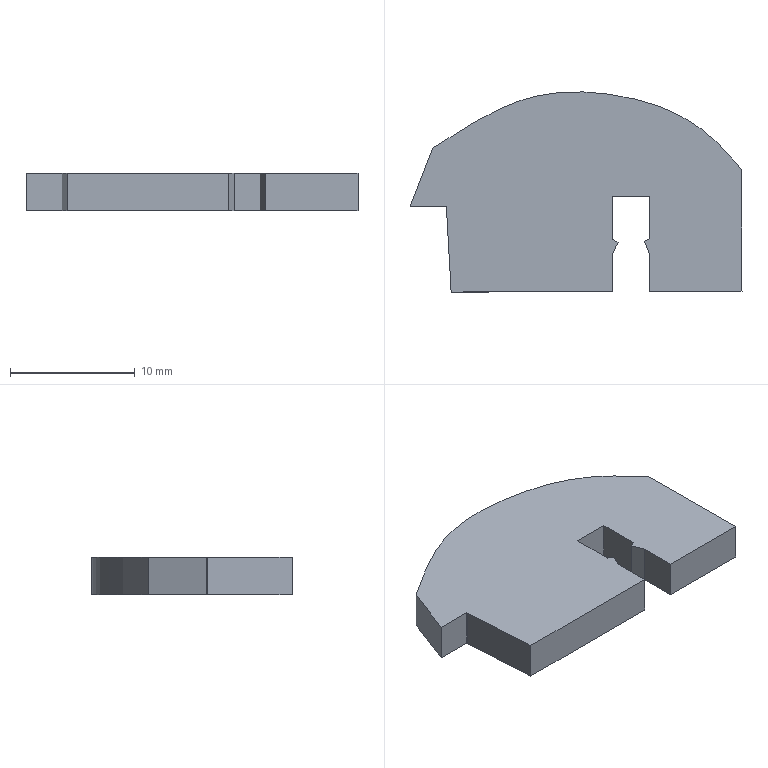Part | SolidWorks | features BaseBody 1 | 1 solid | 22 faces | box 26.661 x 16.081 x 3 mm | volume 988.736 mm3 | plane 18 | spline 4
STEP:
#1=CARTESIAN_POINT('',(-14.881,12.025,-1.5));
#2=VERTEX_POINT('',#1);
#3=CARTESIAN_POINT('',(3.409,15.368,-1.5));
#4=VERTEX_POINT('',#3);
#5=CARTESIAN_POINT('',(-14.881,12.025,-1.5));
#6=CARTESIAN_POINT('',(-13.6,12.857,-1.5));
#7=CARTESIAN_POINT('',(-11.174,14.43,-1.5));
#8=CARTESIAN_POINT('',(-7.153,16.329,-1.5));
#9=CARTESIAN_POINT('',(-3.062,16.713,-1.5));
#10=CARTESIAN_POINT('',(0.49,16.226,-1.5));
#11=CARTESIAN_POINT('',(2.53,15.689,-1.5));
#12=CARTESIAN_POINT('',(3.409,15.368,-1.5));
#13=B_SPLINE_CURVE_WITH_KNOTS('',3,(#5,#6,#7,#8,#9,#10,#11,#12),.UNSPECIFIED.,.F.,.F.,(4,1,1,1,1,4),(0.,0.1649,0.3121,0.4748,0.5989,0.6993),.UNSPECIFIED.);
#14=EDGE_CURVE('',#2,#4,#13,.T.);
#15=ORIENTED_EDGE('',*,*,#14,.T.);
#16=CARTESIAN_POINT('',(6.854,13.453,-1.5));
#17=VERTEX_POINT('',#16);
#18=CARTESIAN_POINT('',(3.409,15.368,-1.5));
#19=CARTESIAN_POINT('',(4.709,14.846,-1.5));
#20=CARTESIAN_POINT('',(5.851,14.197,-1.5));
#21=CARTESIAN_POINT('',(6.854,13.453,-1.5));
#22=B_SPLINE_CURVE_WITH_KNOTS('',3,(#18,#19,#20,#21),.UNSPECIFIED.,.F.,.F.,(4,4),(0.3481,0.3787),.UNSPECIFIED.);
#23=EDGE_CURVE('',#4,#17,#22,.T.);
#24=ORIENTED_EDGE('',*,*,#23,.T.);
#25=CARTESIAN_POINT('',(9.939,10.3,-1.5));
#26=VERTEX_POINT('',#25);
#27=CARTESIAN_POINT('',(6.854,13.453,-1.5));
#28=CARTESIAN_POINT('',(7.525,12.921,-1.5));
#29=CARTESIAN_POINT('',(8.599,11.893,-1.5));
#30=CARTESIAN_POINT('',(9.543,10.77,-1.5));
#31=CARTESIAN_POINT('',(9.939,10.3,-1.5));
#32=B_SPLINE_CURVE_WITH_KNOTS('',3,(#27,#28,#29,#30,#31),.UNSPECIFIED.,.F.,.F.,(4,1,4),(0.8416,0.9336,1.),.UNSPECIFIED.);
#33=EDGE_CURVE('',#17,#26,#32,.T.);
#34=ORIENTED_EDGE('',*,*,#33,.T.);
#35=CARTESIAN_POINT('',(9.963,0.5387,-1.5));
#36=VERTEX_POINT('',#35);
#37=CARTESIAN_POINT('',(9.965,0.02536,-1.5));
#38=DIRECTION('',(-0.002545,1.,0.));
#39=VECTOR('',#38,1000.);
#40=LINE('',#37,#39);
#41=EDGE_CURVE('',#36,#26,#40,.T.);
#42=ORIENTED_EDGE('',*,*,#41,.F.);
#43=CARTESIAN_POINT('',(2.555,0.5198,-1.5));
#44=VERTEX_POINT('',#43);
#45=CARTESIAN_POINT('',(-0.001307,0.5133,-1.5));
#46=DIRECTION('',(1.,0.002545,0.));
#47=VECTOR('',#46,1000.);
#48=LINE('',#45,#47);
#49=EDGE_CURVE('',#44,#36,#48,.T.);
#50=ORIENTED_EDGE('',*,*,#49,.F.);
#51=CARTESIAN_POINT('',(2.555,3.515,-1.5));
#52=VERTEX_POINT('',#51);
#53=CARTESIAN_POINT('',(2.555,0.,-1.5));
#54=DIRECTION('',(0.,-1.,0.));
#55=VECTOR('',#54,1000.);
#56=LINE('',#53,#55);
#57=EDGE_CURVE('',#52,#44,#56,.T.);
#58=ORIENTED_EDGE('',*,*,#57,.F.);
#59=CARTESIAN_POINT('',(2.106,4.558,-1.5));
#60=VERTEX_POINT('',#59);
#61=CARTESIAN_POINT('',(3.432,1.477,-1.5));
#62=DIRECTION('',(0.3953,-0.9186,0.));
#63=VECTOR('',#62,1000.);
#64=LINE('',#61,#63);
#65=EDGE_CURVE('',#60,#52,#64,.T.);
#66=ORIENTED_EDGE('',*,*,#65,.F.);
#67=CARTESIAN_POINT('',(2.555,4.753,-1.5));
#68=VERTEX_POINT('',#67);
#69=CARTESIAN_POINT('',(-1.333,3.06,-1.5));
#70=DIRECTION('',(-0.9168,-0.3993,0.));
#71=VECTOR('',#70,1000.);
#72=LINE('',#69,#71);
#73=EDGE_CURVE('',#68,#60,#72,.T.);
#74=ORIENTED_EDGE('',*,*,#73,.F.);
#75=CARTESIAN_POINT('',(2.555,8.123,-1.5));
#76=VERTEX_POINT('',#75);
#77=CARTESIAN_POINT('',(2.555,0.,-1.5));
#78=DIRECTION('',(0.,-1.,0.));
#79=VECTOR('',#78,1000.);
#80=LINE('',#77,#79);
#81=EDGE_CURVE('',#76,#68,#80,.T.);
#82=ORIENTED_EDGE('',*,*,#81,.F.);
#83=CARTESIAN_POINT('',(-0.4409,8.123,-1.5));
#84=VERTEX_POINT('',#83);
#85=CARTESIAN_POINT('',(0.,8.123,-1.5));
#86=DIRECTION('',(1.,0.,0.));
#87=VECTOR('',#86,1000.);
#88=LINE('',#85,#87);
#89=EDGE_CURVE('',#84,#76,#88,.T.);
#90=ORIENTED_EDGE('',*,*,#89,.F.);
#91=CARTESIAN_POINT('',(-0.4409,4.72,-1.5));
#92=VERTEX_POINT('',#91);
#93=CARTESIAN_POINT('',(-0.4409,0.,-1.5));
#94=DIRECTION('',(0.,1.,0.));
#95=VECTOR('',#94,1000.);
#96=LINE('',#93,#95);
#97=EDGE_CURVE('',#92,#84,#96,.T.);
#98=ORIENTED_EDGE('',*,*,#97,.F.);
#99=CARTESIAN_POINT('',(0.008047,4.456,-1.5));
#100=VERTEX_POINT('',#99);
#101=CARTESIAN_POINT('',(1.952,3.31,-1.5));
#102=DIRECTION('',(-0.8614,0.5079,0.));
#103=VECTOR('',#102,1000.);
#104=LINE('',#101,#103);
#105=EDGE_CURVE('',#100,#92,#104,.T.);
#106=ORIENTED_EDGE('',*,*,#105,.F.);
#107=CARTESIAN_POINT('',(-0.4409,3.497,-1.5));
#108=VERTEX_POINT('',#107);
#109=CARTESIAN_POINT('',(-1.705,0.7988,-1.5));
#110=DIRECTION('',(0.4242,0.9056,0.));
#111=VECTOR('',#110,1000.);
#112=LINE('',#109,#111);
#113=EDGE_CURVE('',#108,#100,#112,.T.);
#114=ORIENTED_EDGE('',*,*,#113,.F.);
#115=CARTESIAN_POINT('',(-0.4409,0.5122,-1.5));
#116=VERTEX_POINT('',#115);
#117=CARTESIAN_POINT('',(-0.4409,0.,-1.5));
#118=DIRECTION('',(0.,1.,0.));
#119=VECTOR('',#118,1000.);
#120=LINE('',#117,#119);
#121=EDGE_CURVE('',#116,#108,#120,.T.);
#122=ORIENTED_EDGE('',*,*,#121,.F.);
#123=CARTESIAN_POINT('',(-13.391,0.4792,-1.5));
#124=VERTEX_POINT('',#123);
#125=CARTESIAN_POINT('',(-0.001307,0.5133,-1.5));
#126=DIRECTION('',(1.,0.002545,0.));
#127=VECTOR('',#126,1000.);
#128=LINE('',#125,#127);
#129=EDGE_CURVE('',#124,#116,#128,.T.);
#130=ORIENTED_EDGE('',*,*,#129,.F.);
#131=CARTESIAN_POINT('',(-13.776,7.259,-1.5));
#132=VERTEX_POINT('',#131);
#133=CARTESIAN_POINT('',(-13.321,-0.7553,-1.5));
#134=DIRECTION('',(0.05661,-0.9984,0.));
#135=VECTOR('',#134,1000.);
#136=LINE('',#133,#135);
#137=EDGE_CURVE('',#132,#124,#136,.T.);
#138=ORIENTED_EDGE('',*,*,#137,.F.);
#139=CARTESIAN_POINT('',(-13.785,7.259,-1.5));
#140=VERTEX_POINT('',#139);
#141=CARTESIAN_POINT('',(-0.01857,7.294,-1.5));
#142=DIRECTION('',(1.,0.002545,0.));
#143=VECTOR('',#142,1000.);
#144=LINE('',#141,#143);
#145=EDGE_CURVE('',#140,#132,#144,.T.);
#146=ORIENTED_EDGE('',*,*,#145,.F.);
#147=CARTESIAN_POINT('',(-13.789,7.354,-1.5));
#148=VERTEX_POINT('',#147);
#149=CARTESIAN_POINT('',(-13.785,7.259,-1.5));
#150=CARTESIAN_POINT('',(-13.786,7.29,-1.5));
#151=CARTESIAN_POINT('',(-13.787,7.322,-1.5));
#152=CARTESIAN_POINT('',(-13.789,7.354,-1.5));
#153=B_SPLINE_CURVE_WITH_KNOTS('',3,(#149,#150,#151,#152),.UNSPECIFIED.,.F.,.F.,(4,4),(0.08216,0.08333),.UNSPECIFIED.);
#154=EDGE_CURVE('',#140,#148,#153,.T.);
#155=ORIENTED_EDGE('',*,*,#154,.T.);
#156=CARTESIAN_POINT('',(-16.697,7.354,-1.5));
#157=VERTEX_POINT('',#156);
#158=CARTESIAN_POINT('',(0.,7.354,-1.5));
#159=DIRECTION('',(-1.,0.,0.));
#160=VECTOR('',#159,1000.);
#161=LINE('',#158,#160);
#162=EDGE_CURVE('',#148,#157,#161,.T.);
#163=ORIENTED_EDGE('',*,*,#162,.T.);
#164=CARTESIAN_POINT('',(-16.988,6.605,-1.5));
#165=DIRECTION('',(-0.3624,-0.932,0.));
#166=VECTOR('',#165,1000.);
#167=LINE('',#164,#166);
#168=EDGE_CURVE('',#2,#157,#167,.T.);
#169=ORIENTED_EDGE('',*,*,#168,.F.);
#170=EDGE_LOOP('',(#15,#24,#34,#42,#50,#58,#66,#74,#82,#90,#98,#106,#114,#122,#130,#138,#146,#155,#163,#169));
#171=FACE_OUTER_BOUND('',#170,.T.);
#172=CARTESIAN_POINT('',(0.,0.,-1.5));
#173=DIRECTION('',(0.,0.,1.));
#174=DIRECTION('',(1.,0.,0.));
#175=AXIS2_PLACEMENT_3D('',#172,#173,#174);
#176=PLANE('',#175);
#177=ADVANCED_FACE('',(#171),#176,.F.);
#178=CARTESIAN_POINT('',(-14.881,12.025,1.5));
#179=VERTEX_POINT('',#178);
#180=CARTESIAN_POINT('',(3.409,15.368,1.5));
#181=VERTEX_POINT('',#180);
#182=CARTESIAN_POINT('',(-14.881,12.025,1.5));
#183=CARTESIAN_POINT('',(-13.6,12.857,1.5));
#184=CARTESIAN_POINT('',(-11.174,14.43,1.5));
#185=CARTESIAN_POINT('',(-7.153,16.329,1.5));
#186=CARTESIAN_POINT('',(-3.062,16.713,1.5));
#187=CARTESIAN_POINT('',(0.49,16.226,1.5));
#188=CARTESIAN_POINT('',(2.53,15.689,1.5));
#189=CARTESIAN_POINT('',(3.409,15.368,1.5));
#190=B_SPLINE_CURVE_WITH_KNOTS('',3,(#182,#183,#184,#185,#186,#187,#188,#189),.UNSPECIFIED.,.F.,.F.,(4,1,1,1,1,4),(0.,0.1649,0.3121,0.4748,0.5989,0.6993),.UNSPECIFIED.);
#191=EDGE_CURVE('',#179,#181,#190,.T.);
#192=ORIENTED_EDGE('',*,*,#191,.F.);
#193=CARTESIAN_POINT('',(-16.697,7.354,1.5));
#194=VERTEX_POINT('',#193);
#195=CARTESIAN_POINT('',(-16.988,6.605,1.5));
#196=DIRECTION('',(-0.3624,-0.932,0.));
#197=VECTOR('',#196,1000.);
#198=LINE('',#195,#197);
#199=EDGE_CURVE('',#179,#194,#198,.T.);
#200=ORIENTED_EDGE('',*,*,#199,.T.);
#201=CARTESIAN_POINT('',(-13.789,7.354,1.5));
#202=VERTEX_POINT('',#201);
#203=CARTESIAN_POINT('',(0.,7.354,1.5));
#204=DIRECTION('',(-1.,0.,0.));
#205=VECTOR('',#204,1000.);
#206=LINE('',#203,#205);
#207=EDGE_CURVE('',#202,#194,#206,.T.);
#208=ORIENTED_EDGE('',*,*,#207,.F.);
#209=CARTESIAN_POINT('',(-13.785,7.259,1.5));
#210=VERTEX_POINT('',#209);
#211=CARTESIAN_POINT('',(-13.785,7.259,1.5));
#212=CARTESIAN_POINT('',(-13.786,7.29,1.5));
#213=CARTESIAN_POINT('',(-13.787,7.322,1.5));
#214=CARTESIAN_POINT('',(-13.789,7.354,1.5));
#215=B_SPLINE_CURVE_WITH_KNOTS('',3,(#211,#212,#213,#214),.UNSPECIFIED.,.F.,.F.,(4,4),(0.08216,0.08333),.UNSPECIFIED.);
#216=EDGE_CURVE('',#210,#202,#215,.T.);
#217=ORIENTED_EDGE('',*,*,#216,.F.);
#218=CARTESIAN_POINT('',(-13.776,7.259,1.5));
#219=VERTEX_POINT('',#218);
#220=CARTESIAN_POINT('',(-0.01857,7.294,1.5));
#221=DIRECTION('',(1.,0.002545,0.));
#222=VECTOR('',#221,1000.);
#223=LINE('',#220,#222);
#224=EDGE_CURVE('',#210,#219,#223,.T.);
#225=ORIENTED_EDGE('',*,*,#224,.T.);
#226=CARTESIAN_POINT('',(-13.391,0.4792,1.5));
#227=VERTEX_POINT('',#226);
#228=CARTESIAN_POINT('',(-13.321,-0.7553,1.5));
#229=DIRECTION('',(0.05661,-0.9984,0.));
#230=VECTOR('',#229,1000.);
#231=LINE('',#228,#230);
#232=EDGE_CURVE('',#219,#227,#231,.T.);
#233=ORIENTED_EDGE('',*,*,#232,.T.);
#234=CARTESIAN_POINT('',(-0.4409,0.5122,1.5));
#235=VERTEX_POINT('',#234);
#236=CARTESIAN_POINT('',(-0.001307,0.5133,1.5));
#237=DIRECTION('',(1.,0.002545,0.));
#238=VECTOR('',#237,1000.);
#239=LINE('',#236,#238);
#240=EDGE_CURVE('',#227,#235,#239,.T.);
#241=ORIENTED_EDGE('',*,*,#240,.T.);
#242=CARTESIAN_POINT('',(-0.4409,3.497,1.5));
#243=VERTEX_POINT('',#242);
#244=CARTESIAN_POINT('',(-0.4409,0.,1.5));
#245=DIRECTION('',(0.,1.,0.));
#246=VECTOR('',#245,1000.);
#247=LINE('',#244,#246);
#248=EDGE_CURVE('',#235,#243,#247,.T.);
#249=ORIENTED_EDGE('',*,*,#248,.T.);
#250=CARTESIAN_POINT('',(0.008047,4.456,1.5));
#251=VERTEX_POINT('',#250);
#252=CARTESIAN_POINT('',(-1.705,0.7988,1.5));
#253=DIRECTION('',(0.4242,0.9056,0.));
#254=VECTOR('',#253,1000.);
#255=LINE('',#252,#254);
#256=EDGE_CURVE('',#243,#251,#255,.T.);
#257=ORIENTED_EDGE('',*,*,#256,.T.);
#258=CARTESIAN_POINT('',(-0.4409,4.72,1.5));
#259=VERTEX_POINT('',#258);
#260=CARTESIAN_POINT('',(1.952,3.31,1.5));
#261=DIRECTION('',(-0.8614,0.5079,0.));
#262=VECTOR('',#261,1000.);
#263=LINE('',#260,#262);
#264=EDGE_CURVE('',#251,#259,#263,.T.);
#265=ORIENTED_EDGE('',*,*,#264,.T.);
#266=CARTESIAN_POINT('',(-0.4409,8.123,1.5));
#267=VERTEX_POINT('',#266);
#268=CARTESIAN_POINT('',(-0.4409,0.,1.5));
#269=DIRECTION('',(0.,1.,0.));
#270=VECTOR('',#269,1000.);
#271=LINE('',#268,#270);
#272=EDGE_CURVE('',#259,#267,#271,.T.);
#273=ORIENTED_EDGE('',*,*,#272,.T.);
#274=CARTESIAN_POINT('',(2.555,8.123,1.5));
#275=VERTEX_POINT('',#274);
#276=CARTESIAN_POINT('',(0.,8.123,1.5));
#277=DIRECTION('',(1.,0.,0.));
#278=VECTOR('',#277,1000.);
#279=LINE('',#276,#278);
#280=EDGE_CURVE('',#267,#275,#279,.T.);
#281=ORIENTED_EDGE('',*,*,#280,.T.);
#282=CARTESIAN_POINT('',(2.555,4.753,1.5));
#283=VERTEX_POINT('',#282);
#284=CARTESIAN_POINT('',(2.555,0.,1.5));
#285=DIRECTION('',(0.,-1.,0.));
#286=VECTOR('',#285,1000.);
#287=LINE('',#284,#286);
#288=EDGE_CURVE('',#275,#283,#287,.T.);
#289=ORIENTED_EDGE('',*,*,#288,.T.);
#290=CARTESIAN_POINT('',(2.106,4.558,1.5));
#291=VERTEX_POINT('',#290);
#292=CARTESIAN_POINT('',(-1.333,3.06,1.5));
#293=DIRECTION('',(-0.9168,-0.3993,0.));
#294=VECTOR('',#293,1000.);
#295=LINE('',#292,#294);
#296=EDGE_CURVE('',#283,#291,#295,.T.);
#297=ORIENTED_EDGE('',*,*,#296,.T.);
#298=CARTESIAN_POINT('',(2.555,3.515,1.5));
#299=VERTEX_POINT('',#298);
#300=CARTESIAN_POINT('',(3.432,1.477,1.5));
#301=DIRECTION('',(0.3953,-0.9186,0.));
#302=VECTOR('',#301,1000.);
#303=LINE('',#300,#302);
#304=EDGE_CURVE('',#291,#299,#303,.T.);
#305=ORIENTED_EDGE('',*,*,#304,.T.);
#306=CARTESIAN_POINT('',(2.555,0.5198,1.5));
#307=VERTEX_POINT('',#306);
#308=CARTESIAN_POINT('',(2.555,0.,1.5));
#309=DIRECTION('',(0.,-1.,0.));
#310=VECTOR('',#309,1000.);
#311=LINE('',#308,#310);
#312=EDGE_CURVE('',#299,#307,#311,.T.);
#313=ORIENTED_EDGE('',*,*,#312,.T.);
#314=CARTESIAN_POINT('',(9.963,0.5387,1.5));
#315=VERTEX_POINT('',#314);
#316=CARTESIAN_POINT('',(-0.001307,0.5133,1.5));
#317=DIRECTION('',(1.,0.002545,0.));
#318=VECTOR('',#317,1000.);
#319=LINE('',#316,#318);
#320=EDGE_CURVE('',#307,#315,#319,.T.);
#321=ORIENTED_EDGE('',*,*,#320,.T.);
#322=CARTESIAN_POINT('',(9.939,10.3,1.5));
#323=VERTEX_POINT('',#322);
#324=CARTESIAN_POINT('',(9.965,0.02536,1.5));
#325=DIRECTION('',(-0.002545,1.,0.));
#326=VECTOR('',#325,1000.);
#327=LINE('',#324,#326);
#328=EDGE_CURVE('',#315,#323,#327,.T.);
#329=ORIENTED_EDGE('',*,*,#328,.T.);
#330=CARTESIAN_POINT('',(6.854,13.453,1.5));
#331=VERTEX_POINT('',#330);
#332=CARTESIAN_POINT('',(6.854,13.453,1.5));
#333=CARTESIAN_POINT('',(7.525,12.921,1.5));
#334=CARTESIAN_POINT('',(8.599,11.893,1.5));
#335=CARTESIAN_POINT('',(9.543,10.77,1.5));
#336=CARTESIAN_POINT('',(9.939,10.3,1.5));
#337=B_SPLINE_CURVE_WITH_KNOTS('',3,(#332,#333,#334,#335,#336),.UNSPECIFIED.,.F.,.F.,(4,1,4),(0.8416,0.9336,1.),.UNSPECIFIED.);
#338=EDGE_CURVE('',#331,#323,#337,.T.);
#339=ORIENTED_EDGE('',*,*,#338,.F.);
#340=CARTESIAN_POINT('',(3.409,15.368,1.5));
#341=CARTESIAN_POINT('',(4.709,14.846,1.5));
#342=CARTESIAN_POINT('',(5.851,14.197,1.5));
#343=CARTESIAN_POINT('',(6.854,13.453,1.5));
#344=B_SPLINE_CURVE_WITH_KNOTS('',3,(#340,#341,#342,#343),.UNSPECIFIED.,.F.,.F.,(4,4),(0.3481,0.3787),.UNSPECIFIED.);
#345=EDGE_CURVE('',#181,#331,#344,.T.);
#346=ORIENTED_EDGE('',*,*,#345,.F.);
#347=EDGE_LOOP('',(#192,#200,#208,#217,#225,#233,#241,#249,#257,#265,#273,#281,#289,#297,#305,#313,#321,#329,#339,#346));
#348=FACE_OUTER_BOUND('',#347,.T.);
#349=CARTESIAN_POINT('',(0.,0.,1.5));
#350=DIRECTION('',(0.,0.,1.));
#351=DIRECTION('',(1.,0.,0.));
#352=AXIS2_PLACEMENT_3D('',#349,#350,#351);
#353=PLANE('',#352);
#354=ADVANCED_FACE('',(#348),#353,.T.);
#355=ORIENTED_EDGE('',*,*,#23,.F.);
#356=CARTESIAN_POINT('',(3.409,15.368,1.5));
#357=DIRECTION('',(0.,0.,-1.));
#358=VECTOR('',#357,1000.);
#359=LINE('',#356,#358);
#360=EDGE_CURVE('',#181,#4,#359,.T.);
#361=ORIENTED_EDGE('',*,*,#360,.F.);
#362=ORIENTED_EDGE('',*,*,#345,.T.);
#363=CARTESIAN_POINT('',(6.854,13.453,1.5));
#364=DIRECTION('',(0.,0.,-1.));
#365=VECTOR('',#364,1000.);
#366=LINE('',#363,#365);
#367=EDGE_CURVE('',#331,#17,#366,.T.);
#368=ORIENTED_EDGE('',*,*,#367,.T.);
#369=EDGE_LOOP('',(#355,#361,#362,#368));
#370=FACE_OUTER_BOUND('',#369,.T.);
#371=CARTESIAN_POINT('',(3.409,15.368,1.5));
#372=CARTESIAN_POINT('',(3.409,15.368,-1.5));
#373=CARTESIAN_POINT('',(4.709,14.846,1.5));
#374=CARTESIAN_POINT('',(4.709,14.846,-1.5));
#375=CARTESIAN_POINT('',(5.851,14.197,1.5));
#376=CARTESIAN_POINT('',(5.851,14.197,-1.5));
#377=CARTESIAN_POINT('',(6.854,13.453,1.5));
#378=CARTESIAN_POINT('',(6.854,13.453,-1.5));
#379=B_SPLINE_SURFACE_WITH_KNOTS('',3,1,((#371,#372),(#373,#374),(#375,#376),(#377,#378)),.UNSPECIFIED.,.F.,.F.,.F.,(4,4),(2,2),(0.3481,0.3787),(0.,1.),.UNSPECIFIED.);
#380=ADVANCED_FACE('',(#370),#379,.T.);
#381=ORIENTED_EDGE('',*,*,#33,.F.);
#382=ORIENTED_EDGE('',*,*,#367,.F.);
#383=ORIENTED_EDGE('',*,*,#338,.T.);
#384=CARTESIAN_POINT('',(9.939,10.3,1.5));
#385=DIRECTION('',(0.,0.,-1.));
#386=VECTOR('',#385,1000.);
#387=LINE('',#384,#386);
#388=EDGE_CURVE('',#323,#26,#387,.T.);
#389=ORIENTED_EDGE('',*,*,#388,.T.);
#390=EDGE_LOOP('',(#381,#382,#383,#389));
#391=FACE_OUTER_BOUND('',#390,.T.);
#392=CARTESIAN_POINT('',(6.854,13.453,1.5));
#393=CARTESIAN_POINT('',(6.854,13.453,-1.5));
#394=CARTESIAN_POINT('',(7.525,12.921,1.5));
#395=CARTESIAN_POINT('',(7.525,12.921,-1.5));
#396=CARTESIAN_POINT('',(8.599,11.893,1.5));
#397=CARTESIAN_POINT('',(8.599,11.893,-1.5));
#398=CARTESIAN_POINT('',(9.543,10.77,1.5));
#399=CARTESIAN_POINT('',(9.543,10.77,-1.5));
#400=CARTESIAN_POINT('',(9.939,10.3,1.5));
#401=CARTESIAN_POINT('',(9.939,10.3,-1.5));
#402=B_SPLINE_SURFACE_WITH_KNOTS('',3,1,((#392,#393),(#394,#395),(#396,#397),(#398,#399),(#400,#401)),.UNSPECIFIED.,.F.,.F.,.F.,(4,1,4),(2,2),(0.8416,0.9336,1.),(0.,1.),.UNSPECIFIED.);
#403=ADVANCED_FACE('',(#391),#402,.T.);
#404=ORIENTED_EDGE('',*,*,#41,.T.);
#405=ORIENTED_EDGE('',*,*,#388,.F.);
#406=ORIENTED_EDGE('',*,*,#328,.F.);
#407=CARTESIAN_POINT('',(9.963,0.5387,1.5));
#408=DIRECTION('',(0.,0.,-1.));
#409=VECTOR('',#408,1000.);
#410=LINE('',#407,#409);
#411=EDGE_CURVE('',#315,#36,#410,.T.);
#412=ORIENTED_EDGE('',*,*,#411,.T.);
#413=EDGE_LOOP('',(#404,#405,#406,#412));
#414=FACE_OUTER_BOUND('',#413,.T.);
#415=CARTESIAN_POINT('',(9.965,0.02536,1.5));
#416=DIRECTION('',(-1.,-0.002545,0.));
#417=DIRECTION('',(-0.002545,1.,0.));
#418=AXIS2_PLACEMENT_3D('',#415,#416,#417);
#419=PLANE('',#418);
#420=ADVANCED_FACE('',(#414),#419,.F.);
#421=ORIENTED_EDGE('',*,*,#49,.T.);
#422=ORIENTED_EDGE('',*,*,#411,.F.);
#423=ORIENTED_EDGE('',*,*,#320,.F.);
#424=CARTESIAN_POINT('',(2.555,0.5198,1.5));
#425=DIRECTION('',(0.,0.,-1.));
#426=VECTOR('',#425,1000.);
#427=LINE('',#424,#426);
#428=EDGE_CURVE('',#307,#44,#427,.T.);
#429=ORIENTED_EDGE('',*,*,#428,.T.);
#430=EDGE_LOOP('',(#421,#422,#423,#429));
#431=FACE_OUTER_BOUND('',#430,.T.);
#432=CARTESIAN_POINT('',(-0.001307,0.5133,1.5));
#433=DIRECTION('',(-0.002545,1.,0.));
#434=DIRECTION('',(0.,0.,1.));
#435=AXIS2_PLACEMENT_3D('',#432,#433,#434);
#436=PLANE('',#435);
#437=ADVANCED_FACE('',(#431),#436,.F.);
#438=ORIENTED_EDGE('',*,*,#57,.T.);
#439=ORIENTED_EDGE('',*,*,#428,.F.);
#440=ORIENTED_EDGE('',*,*,#312,.F.);
#441=CARTESIAN_POINT('',(2.555,3.515,1.5));
#442=DIRECTION('',(0.,0.,-1.));
#443=VECTOR('',#442,1000.);
#444=LINE('',#441,#443);
#445=EDGE_CURVE('',#299,#52,#444,.T.);
#446=ORIENTED_EDGE('',*,*,#445,.T.);
#447=EDGE_LOOP('',(#438,#439,#440,#446));
#448=FACE_OUTER_BOUND('',#447,.T.);
#449=CARTESIAN_POINT('',(2.555,0.,1.5));
#450=DIRECTION('',(1.,0.,0.));
#451=DIRECTION('',(0.,1.,0.));
#452=AXIS2_PLACEMENT_3D('',#449,#450,#451);
#453=PLANE('',#452);
#454=ADVANCED_FACE('',(#448),#453,.F.);
#455=ORIENTED_EDGE('',*,*,#65,.T.);
#456=ORIENTED_EDGE('',*,*,#445,.F.);
#457=ORIENTED_EDGE('',*,*,#304,.F.);
#458=CARTESIAN_POINT('',(2.106,4.558,1.5));
#459=DIRECTION('',(0.,0.,-1.));
#460=VECTOR('',#459,1000.);
#461=LINE('',#458,#460);
#462=EDGE_CURVE('',#291,#60,#461,.T.);
#463=ORIENTED_EDGE('',*,*,#462,.T.);
#464=EDGE_LOOP('',(#455,#456,#457,#463));
#465=FACE_OUTER_BOUND('',#464,.T.);
#466=CARTESIAN_POINT('',(3.432,1.477,1.5));
#467=DIRECTION('',(0.9186,0.3953,0.));
#468=DIRECTION('',(0.,0.,-1.));
#469=AXIS2_PLACEMENT_3D('',#466,#467,#468);
#470=PLANE('',#469);
#471=ADVANCED_FACE('',(#465),#470,.F.);
#472=ORIENTED_EDGE('',*,*,#73,.T.);
#473=ORIENTED_EDGE('',*,*,#462,.F.);
#474=ORIENTED_EDGE('',*,*,#296,.F.);
#475=CARTESIAN_POINT('',(2.555,4.753,1.5));
#476=DIRECTION('',(0.,0.,-1.));
#477=VECTOR('',#476,1000.);
#478=LINE('',#475,#477);
#479=EDGE_CURVE('',#283,#68,#478,.T.);
#480=ORIENTED_EDGE('',*,*,#479,.T.);
#481=EDGE_LOOP('',(#472,#473,#474,#480));
#482=FACE_OUTER_BOUND('',#481,.T.);
#483=CARTESIAN_POINT('',(-1.333,3.06,1.5));
#484=DIRECTION('',(0.3993,-0.9168,0.));
#485=DIRECTION('',(0.,0.,-1.));
#486=AXIS2_PLACEMENT_3D('',#483,#484,#485);
#487=PLANE('',#486);
#488=ADVANCED_FACE('',(#482),#487,.F.);
#489=ORIENTED_EDGE('',*,*,#81,.T.);
#490=ORIENTED_EDGE('',*,*,#479,.F.);
#491=ORIENTED_EDGE('',*,*,#288,.F.);
#492=CARTESIAN_POINT('',(2.555,8.123,1.5));
#493=DIRECTION('',(0.,0.,-1.));
#494=VECTOR('',#493,1000.);
#495=LINE('',#492,#494);
#496=EDGE_CURVE('',#275,#76,#495,.T.);
#497=ORIENTED_EDGE('',*,*,#496,.T.);
#498=EDGE_LOOP('',(#489,#490,#491,#497));
#499=FACE_OUTER_BOUND('',#498,.T.);
#500=CARTESIAN_POINT('',(2.555,0.,1.5));
#501=DIRECTION('',(1.,0.,0.));
#502=DIRECTION('',(0.,1.,0.));
#503=AXIS2_PLACEMENT_3D('',#500,#501,#502);
#504=PLANE('',#503);
#505=ADVANCED_FACE('',(#499),#504,.F.);
#506=ORIENTED_EDGE('',*,*,#89,.T.);
#507=ORIENTED_EDGE('',*,*,#496,.F.);
#508=ORIENTED_EDGE('',*,*,#280,.F.);
#509=CARTESIAN_POINT('',(-0.4409,8.123,1.5));
#510=DIRECTION('',(0.,0.,-1.));
#511=VECTOR('',#510,1000.);
#512=LINE('',#509,#511);
#513=EDGE_CURVE('',#267,#84,#512,.T.);
#514=ORIENTED_EDGE('',*,*,#513,.T.);
#515=EDGE_LOOP('',(#506,#507,#508,#514));
#516=FACE_OUTER_BOUND('',#515,.T.);
#517=CARTESIAN_POINT('',(0.,8.123,1.5));
#518=DIRECTION('',(0.,1.,0.));
#519=DIRECTION('',(1.,0.,0.));
#520=AXIS2_PLACEMENT_3D('',#517,#518,#519);
#521=PLANE('',#520);
#522=ADVANCED_FACE('',(#516),#521,.F.);
#523=ORIENTED_EDGE('',*,*,#97,.T.);
#524=ORIENTED_EDGE('',*,*,#513,.F.);
#525=ORIENTED_EDGE('',*,*,#272,.F.);
#526=CARTESIAN_POINT('',(-0.4409,4.72,1.5));
#527=DIRECTION('',(0.,0.,-1.));
#528=VECTOR('',#527,1000.);
#529=LINE('',#526,#528);
#530=EDGE_CURVE('',#259,#92,#529,.T.);
#531=ORIENTED_EDGE('',*,*,#530,.T.);
#532=EDGE_LOOP('',(#523,#524,#525,#531));
#533=FACE_OUTER_BOUND('',#532,.T.);
#534=CARTESIAN_POINT('',(-0.4409,0.,1.5));
#535=DIRECTION('',(-1.,0.,0.));
#536=DIRECTION('',(0.,0.,1.));
#537=AXIS2_PLACEMENT_3D('',#534,#535,#536);
#538=PLANE('',#537);
#539=ADVANCED_FACE('',(#533),#538,.F.);
#540=ORIENTED_EDGE('',*,*,#105,.T.);
#541=ORIENTED_EDGE('',*,*,#530,.F.);
#542=ORIENTED_EDGE('',*,*,#264,.F.);
#543=CARTESIAN_POINT('',(0.008047,4.456,1.5));
#544=DIRECTION('',(0.,0.,-1.));
#545=VECTOR('',#544,1000.);
#546=LINE('',#543,#545);
#547=EDGE_CURVE('',#251,#100,#546,.T.);
#548=ORIENTED_EDGE('',*,*,#547,.T.);
#549=EDGE_LOOP('',(#540,#541,#542,#548));
#550=FACE_OUTER_BOUND('',#549,.T.);
#551=CARTESIAN_POINT('',(1.952,3.31,1.5));
#552=DIRECTION('',(-0.5079,-0.8614,0.));
#553=DIRECTION('',(-0.8614,0.5079,0.));
#554=AXIS2_PLACEMENT_3D('',#551,#552,#553);
#555=PLANE('',#554);
#556=ADVANCED_FACE('',(#550),#555,.F.);
#557=ORIENTED_EDGE('',*,*,#113,.T.);
#558=ORIENTED_EDGE('',*,*,#547,.F.);
#559=ORIENTED_EDGE('',*,*,#256,.F.);
#560=CARTESIAN_POINT('',(-0.4409,3.497,1.5));
#561=DIRECTION('',(0.,0.,-1.));
#562=VECTOR('',#561,1000.);
#563=LINE('',#560,#562);
#564=EDGE_CURVE('',#243,#108,#563,.T.);
#565=ORIENTED_EDGE('',*,*,#564,.T.);
#566=EDGE_LOOP('',(#557,#558,#559,#565));
#567=FACE_OUTER_BOUND('',#566,.T.);
#568=CARTESIAN_POINT('',(-1.705,0.7988,1.5));
#569=DIRECTION('',(-0.9056,0.4242,0.));
#570=DIRECTION('',(0.,0.,1.));
#571=AXIS2_PLACEMENT_3D('',#568,#569,#570);
#572=PLANE('',#571);
#573=ADVANCED_FACE('',(#567),#572,.F.);
#574=ORIENTED_EDGE('',*,*,#121,.T.);
#575=ORIENTED_EDGE('',*,*,#564,.F.);
#576=ORIENTED_EDGE('',*,*,#248,.F.);
#577=CARTESIAN_POINT('',(-0.4409,0.5122,1.5));
#578=DIRECTION('',(0.,0.,-1.));
#579=VECTOR('',#578,1000.);
#580=LINE('',#577,#579);
#581=EDGE_CURVE('',#235,#116,#580,.T.);
#582=ORIENTED_EDGE('',*,*,#581,.T.);
#583=EDGE_LOOP('',(#574,#575,#576,#582));
#584=FACE_OUTER_BOUND('',#583,.T.);
#585=CARTESIAN_POINT('',(-0.4409,0.,1.5));
#586=DIRECTION('',(-1.,0.,0.));
#587=DIRECTION('',(0.,0.,1.));
#588=AXIS2_PLACEMENT_3D('',#585,#586,#587);
#589=PLANE('',#588);
#590=ADVANCED_FACE('',(#584),#589,.F.);
#591=ORIENTED_EDGE('',*,*,#129,.T.);
#592=ORIENTED_EDGE('',*,*,#581,.F.);
#593=ORIENTED_EDGE('',*,*,#240,.F.);
#594=CARTESIAN_POINT('',(-13.391,0.4792,1.5));
#595=DIRECTION('',(0.,0.,-1.));
#596=VECTOR('',#595,1000.);
#597=LINE('',#594,#596);
#598=EDGE_CURVE('',#227,#124,#597,.T.);
#599=ORIENTED_EDGE('',*,*,#598,.T.);
#600=EDGE_LOOP('',(#591,#592,#593,#599));
#601=FACE_OUTER_BOUND('',#600,.T.);
#602=CARTESIAN_POINT('',(-0.001307,0.5133,1.5));
#603=DIRECTION('',(-0.002545,1.,0.));
#604=DIRECTION('',(0.,0.,1.));
#605=AXIS2_PLACEMENT_3D('',#602,#603,#604);
#606=PLANE('',#605);
#607=ADVANCED_FACE('',(#601),#606,.F.);
#608=ORIENTED_EDGE('',*,*,#137,.T.);
#609=ORIENTED_EDGE('',*,*,#598,.F.);
#610=ORIENTED_EDGE('',*,*,#232,.F.);
#611=CARTESIAN_POINT('',(-13.776,7.259,1.5));
#612=DIRECTION('',(0.,0.,-1.));
#613=VECTOR('',#612,1000.);
#614=LINE('',#611,#613);
#615=EDGE_CURVE('',#219,#132,#614,.T.);
#616=ORIENTED_EDGE('',*,*,#615,.T.);
#617=EDGE_LOOP('',(#608,#609,#610,#616));
#618=FACE_OUTER_BOUND('',#617,.T.);
#619=CARTESIAN_POINT('',(-13.321,-0.7553,1.5));
#620=DIRECTION('',(0.9984,0.05661,0.));
#621=DIRECTION('',(0.,0.,-1.));
#622=AXIS2_PLACEMENT_3D('',#619,#620,#621);
#623=PLANE('',#622);
#624=ADVANCED_FACE('',(#618),#623,.F.);
#625=ORIENTED_EDGE('',*,*,#145,.T.);
#626=ORIENTED_EDGE('',*,*,#615,.F.);
#627=ORIENTED_EDGE('',*,*,#224,.F.);
#628=CARTESIAN_POINT('',(-13.785,7.259,1.5));
#629=DIRECTION('',(0.,0.,-1.));
#630=VECTOR('',#629,1000.);
#631=LINE('',#628,#630);
#632=EDGE_CURVE('',#210,#140,#631,.T.);
#633=ORIENTED_EDGE('',*,*,#632,.T.);
#634=EDGE_LOOP('',(#625,#626,#627,#633));
#635=FACE_OUTER_BOUND('',#634,.T.);
#636=CARTESIAN_POINT('',(-0.01857,7.294,1.5));
#637=DIRECTION('',(-0.002545,1.,0.));
#638=DIRECTION('',(0.,0.,1.));
#639=AXIS2_PLACEMENT_3D('',#636,#637,#638);
#640=PLANE('',#639);
#641=ADVANCED_FACE('',(#635),#640,.F.);
#642=ORIENTED_EDGE('',*,*,#154,.F.);
#643=ORIENTED_EDGE('',*,*,#632,.F.);
#644=ORIENTED_EDGE('',*,*,#216,.T.);
#645=CARTESIAN_POINT('',(-13.789,7.354,1.5));
#646=DIRECTION('',(0.,0.,-1.));
#647=VECTOR('',#646,1000.);
#648=LINE('',#645,#647);
#649=EDGE_CURVE('',#202,#148,#648,.T.);
#650=ORIENTED_EDGE('',*,*,#649,.T.);
#651=EDGE_LOOP('',(#642,#643,#644,#650));
#652=FACE_OUTER_BOUND('',#651,.T.);
#653=CARTESIAN_POINT('',(-13.785,7.259,1.5));
#654=CARTESIAN_POINT('',(-13.785,7.259,-1.5));
#655=CARTESIAN_POINT('',(-13.786,7.29,1.5));
#656=CARTESIAN_POINT('',(-13.786,7.29,-1.5));
#657=CARTESIAN_POINT('',(-13.787,7.322,1.5));
#658=CARTESIAN_POINT('',(-13.787,7.322,-1.5));
#659=CARTESIAN_POINT('',(-13.789,7.354,1.5));
#660=CARTESIAN_POINT('',(-13.789,7.354,-1.5));
#661=B_SPLINE_SURFACE_WITH_KNOTS('',3,1,((#653,#654),(#655,#656),(#657,#658),(#659,#660)),.UNSPECIFIED.,.F.,.F.,.F.,(4,4),(2,2),(0.08216,0.08333),(0.,1.),.UNSPECIFIED.);
#662=ADVANCED_FACE('',(#652),#661,.T.);
#663=ORIENTED_EDGE('',*,*,#162,.F.);
#664=ORIENTED_EDGE('',*,*,#649,.F.);
#665=ORIENTED_EDGE('',*,*,#207,.T.);
#666=CARTESIAN_POINT('',(-16.697,7.354,1.5));
#667=DIRECTION('',(0.,0.,-1.));
#668=VECTOR('',#667,1000.);
#669=LINE('',#666,#668);
#670=EDGE_CURVE('',#194,#157,#669,.T.);
#671=ORIENTED_EDGE('',*,*,#670,.T.);
#672=EDGE_LOOP('',(#663,#664,#665,#671));
#673=FACE_OUTER_BOUND('',#672,.T.);
#674=CARTESIAN_POINT('',(0.,7.354,1.5));
#675=DIRECTION('',(0.,-1.,0.));
#676=DIRECTION('',(0.,0.,-1.));
#677=AXIS2_PLACEMENT_3D('',#674,#675,#676);
#678=PLANE('',#677);
#679=ADVANCED_FACE('',(#673),#678,.T.);
#680=ORIENTED_EDGE('',*,*,#168,.T.);
#681=ORIENTED_EDGE('',*,*,#670,.F.);
#682=ORIENTED_EDGE('',*,*,#199,.F.);
#683=CARTESIAN_POINT('',(-14.881,12.025,1.5));
#684=DIRECTION('',(0.,0.,-1.));
#685=VECTOR('',#684,1000.);
#686=LINE('',#683,#685);
#687=EDGE_CURVE('',#179,#2,#686,.T.);
#688=ORIENTED_EDGE('',*,*,#687,.T.);
#689=EDGE_LOOP('',(#680,#681,#682,#688));
#690=FACE_OUTER_BOUND('',#689,.T.);
#691=CARTESIAN_POINT('',(-16.988,6.605,1.5));
#692=DIRECTION('',(0.932,-0.3624,0.));
#693=DIRECTION('',(0.,0.,-1.));
#694=AXIS2_PLACEMENT_3D('',#691,#692,#693);
#695=PLANE('',#694);
#696=ADVANCED_FACE('',(#690),#695,.F.);
#697=ORIENTED_EDGE('',*,*,#14,.F.);
#698=ORIENTED_EDGE('',*,*,#687,.F.);
#699=ORIENTED_EDGE('',*,*,#191,.T.);
#700=ORIENTED_EDGE('',*,*,#360,.T.);
#701=EDGE_LOOP('',(#697,#698,#699,#700));
#702=FACE_OUTER_BOUND('',#701,.T.);
#703=CARTESIAN_POINT('',(-14.881,12.025,1.5));
#704=CARTESIAN_POINT('',(-14.881,12.025,-1.5));
#705=CARTESIAN_POINT('',(-13.6,12.857,1.5));
#706=CARTESIAN_POINT('',(-13.6,12.857,-1.5));
#707=CARTESIAN_POINT('',(-11.174,14.43,1.5));
#708=CARTESIAN_POINT('',(-11.174,14.43,-1.5));
#709=CARTESIAN_POINT('',(-7.153,16.329,1.5));
#710=CARTESIAN_POINT('',(-7.153,16.329,-1.5));
#711=CARTESIAN_POINT('',(-3.062,16.713,1.5));
#712=CARTESIAN_POINT('',(-3.062,16.713,-1.5));
#713=CARTESIAN_POINT('',(0.49,16.226,1.5));
#714=CARTESIAN_POINT('',(0.49,16.226,-1.5));
#715=CARTESIAN_POINT('',(2.53,15.689,1.5));
#716=CARTESIAN_POINT('',(2.53,15.689,-1.5));
#717=CARTESIAN_POINT('',(3.409,15.368,1.5));
#718=CARTESIAN_POINT('',(3.409,15.368,-1.5));
#719=B_SPLINE_SURFACE_WITH_KNOTS('',3,1,((#703,#704),(#705,#706),(#707,#708),(#709,#710),(#711,#712),(#713,#714),(#715,#716),(#717,#718)),.UNSPECIFIED.,.F.,.F.,.F.,(4,1,1,1,1,4),(2,2),(0.,0.1649,0.3121,0.4748,0.5989,0.6993),(0.,1.),.UNSPECIFIED.);
#720=ADVANCED_FACE('',(#702),#719,.T.);
#721=CLOSED_SHELL('',(#177,#354,#380,#403,#420,#437,#454,#471,#488,#505,#522,#539,#556,#573,#590,#607,#624,#641,#662,#679,#696,#720));
#722=MANIFOLD_SOLID_BREP('',#721);
#723=CARTESIAN_POINT('',(0.,0.,0.));
#724=DIRECTION('',(0.,0.,1.));
#725=DIRECTION('',(1.,0.,0.));
#726=AXIS2_PLACEMENT_3D('',#723,#724,#725);
#727=(LENGTH_UNIT()NAMED_UNIT(*)SI_UNIT(.MILLI.,.METRE.));
#728=UNCERTAINTY_MEASURE_WITH_UNIT(LENGTH_MEASURE(0.00001),#727,'','');
#729=(NAMED_UNIT(*)PLANE_ANGLE_UNIT()SI_UNIT($,.RADIAN.));
#730=(NAMED_UNIT(*)SI_UNIT($,.STERADIAN.)SOLID_ANGLE_UNIT());
#731=(GEOMETRIC_REPRESENTATION_CONTEXT(3)GLOBAL_UNCERTAINTY_ASSIGNED_CONTEXT((#728))GLOBAL_UNIT_ASSIGNED_CONTEXT((#727,#729,#730))REPRESENTATION_CONTEXT('',''));
#732=ADVANCED_BREP_SHAPE_REPRESENTATION('',(#722,#726),#731);